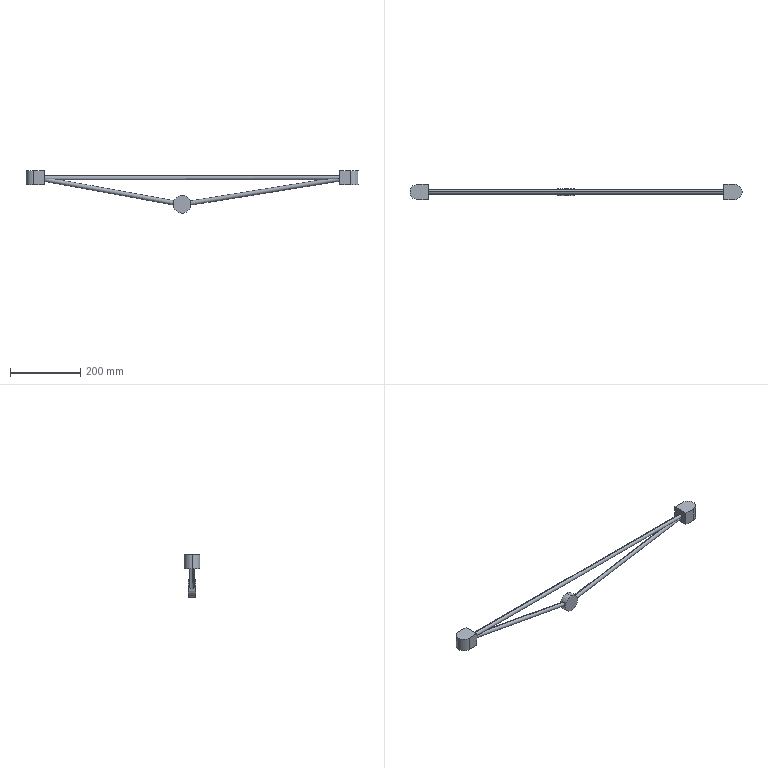Part | SolidWorks | features MoveFace 4, BaseBody 2, Sweep 1 | 1 solid | 23 faces | box 944 x 44 x 120.397 mm | volume 388537 mm3 | plane 12 | cylinder 11 | commonest cylinder face diameters 12 x6 44 x3 50 x2
STEP:
#1=CARTESIAN_POINT('',(546.798,0.,-77.466));
#2=VERTEX_POINT('',#1);
#3=CARTESIAN_POINT('',(544.892,0.,-65.619));
#4=VERTEX_POINT('',#3);
#5=CARTESIAN_POINT('',(546.798,0.,-77.466));
#6=CARTESIAN_POINT('',(546.798,0.398,-77.466));
#7=CARTESIAN_POINT('',(546.801,0.7891,-77.426));
#8=CARTESIAN_POINT('',(546.81,1.366,-77.308));
#9=CARTESIAN_POINT('',(546.814,1.556,-77.259));
#10=CARTESIAN_POINT('',(546.823,1.934,-77.142));
#11=CARTESIAN_POINT('',(546.827,2.121,-77.073));
#12=CARTESIAN_POINT('',(546.842,2.666,-76.841));
#13=CARTESIAN_POINT('',(546.853,3.01,-76.653));
#14=CARTESIAN_POINT('',(546.871,3.661,-76.209));
#15=CARTESIAN_POINT('',(546.879,3.968,-75.952));
#16=CARTESIAN_POINT('',(546.885,4.519,-75.392));
#17=CARTESIAN_POINT('',(546.884,4.767,-75.087));
#18=CARTESIAN_POINT('',(546.867,5.206,-74.426));
#19=CARTESIAN_POINT('',(546.851,5.391,-74.077));
#20=CARTESIAN_POINT('',(546.815,5.616,-73.535));
#21=CARTESIAN_POINT('',(546.8,5.682,-73.351));
#22=CARTESIAN_POINT('',(546.767,5.797,-72.975));
#23=CARTESIAN_POINT('',(546.747,5.845,-72.782));
#24=CARTESIAN_POINT('',(546.682,5.961,-72.204));
#25=CARTESIAN_POINT('',(546.629,6.,-71.817));
#26=CARTESIAN_POINT('',(546.504,6.,-71.041));
#27=CARTESIAN_POINT('',(546.431,5.961,-70.648));
#28=CARTESIAN_POINT('',(546.273,5.807,-69.893));
#29=CARTESIAN_POINT('',(546.187,5.693,-69.527));
#30=CARTESIAN_POINT('',(546.051,5.466,-68.996));
#31=CARTESIAN_POINT('',(546.004,5.381,-68.822));
#32=CARTESIAN_POINT('',(545.91,5.196,-68.486));
#33=CARTESIAN_POINT('',(545.863,5.095,-68.324));
#34=CARTESIAN_POINT('',(545.768,4.878,-68.011));
#35=CARTESIAN_POINT('',(545.721,4.762,-67.86));
#36=CARTESIAN_POINT('',(545.627,4.513,-67.569));
#37=CARTESIAN_POINT('',(545.58,4.381,-67.428));
#38=CARTESIAN_POINT('',(545.443,3.963,-67.027));
#39=CARTESIAN_POINT('',(545.357,3.662,-66.791));
#40=CARTESIAN_POINT('',(545.2,3.013,-66.376));
#41=CARTESIAN_POINT('',(545.13,2.662,-66.197));
#42=CARTESIAN_POINT('',(545.014,1.937,-65.911));
#43=CARTESIAN_POINT('',(544.969,1.563,-65.803));
#44=CARTESIAN_POINT('',(544.923,0.9839,-65.693));
#45=CARTESIAN_POINT('',(544.911,0.7866,-65.665));
#46=CARTESIAN_POINT('',(544.896,0.3928,-65.628));
#47=CARTESIAN_POINT('',(544.892,0.1962,-65.619));
#48=CARTESIAN_POINT('',(544.892,0.,-65.619));
#49=B_SPLINE_CURVE_WITH_KNOTS('',3,(#5,#6,#7,#8,#9,#10,#11,#12,#13,#14,#15,#16,#17,#18,#19,#20,#21,#22,#23,#24,#25,#26,#27,#28,#29,#30,#31,#32,#33,#34,#35,#36,#37,#38,#39,#40,#41,#42,#43,#44,#45,#46,#47,#48),.UNSPECIFIED.,.F.,.F.,(4,2,2,2,2,2,2,2,2,2,2,2,2,2,2,2,2,2,2,2,2,4),(0.,0.001177,0.001765,0.002353,0.00353,0.004707,0.005884,0.00706,0.007649,0.008237,0.009414,0.01059,0.01177,0.01236,0.01294,0.01353,0.01412,0.0153,0.01647,0.01765,0.01824,0.01883),.UNSPECIFIED.);
#50=EDGE_CURVE('',#2,#4,#49,.T.);
#51=ORIENTED_EDGE('',*,*,#50,.F.);
#52=CARTESIAN_POINT('',(544.892,0.,-65.619));
#53=CARTESIAN_POINT('',(544.892,-0.3923,-65.619));
#54=CARTESIAN_POINT('',(544.907,-0.7833,-65.655));
#55=CARTESIAN_POINT('',(544.969,-1.562,-65.802));
#56=CARTESIAN_POINT('',(545.015,-1.938,-65.911));
#57=CARTESIAN_POINT('',(545.101,-2.48,-66.125));
#58=CARTESIAN_POINT('',(545.132,-2.657,-66.205));
#59=CARTESIAN_POINT('',(545.202,-3.004,-66.382));
#60=CARTESIAN_POINT('',(545.239,-3.174,-66.479));
#61=CARTESIAN_POINT('',(545.357,-3.663,-66.791));
#62=CARTESIAN_POINT('',(545.443,-3.964,-67.028));
#63=CARTESIAN_POINT('',(545.625,-4.517,-67.559));
#64=CARTESIAN_POINT('',(545.721,-4.769,-67.854));
#65=CARTESIAN_POINT('',(545.91,-5.203,-68.481));
#66=CARTESIAN_POINT('',(546.004,-5.388,-68.814));
#67=CARTESIAN_POINT('',(546.187,-5.692,-69.523));
#68=CARTESIAN_POINT('',(546.273,-5.807,-69.892));
#69=CARTESIAN_POINT('',(546.391,-5.922,-70.457));
#70=CARTESIAN_POINT('',(546.429,-5.951,-70.647));
#71=CARTESIAN_POINT('',(546.5,-5.99,-71.033));
#72=CARTESIAN_POINT('',(546.534,-6.,-71.229));
#73=CARTESIAN_POINT('',(546.629,-6.,-71.815));
#74=CARTESIAN_POINT('',(546.682,-5.961,-72.202));
#75=CARTESIAN_POINT('',(546.768,-5.808,-72.968));
#76=CARTESIAN_POINT('',(546.802,-5.692,-73.351));
#77=CARTESIAN_POINT('',(546.851,-5.392,-74.076));
#78=CARTESIAN_POINT('',(546.867,-5.208,-74.423));
#79=CARTESIAN_POINT('',(546.879,-4.88,-74.917));
#80=CARTESIAN_POINT('',(546.882,-4.762,-75.078));
#81=CARTESIAN_POINT('',(546.884,-4.513,-75.385));
#82=CARTESIAN_POINT('',(546.884,-4.382,-75.531));
#83=CARTESIAN_POINT('',(546.879,-3.97,-75.95));
#84=CARTESIAN_POINT('',(546.871,-3.666,-76.205));
#85=CARTESIAN_POINT('',(546.853,-3.011,-76.652));
#86=CARTESIAN_POINT('',(546.842,-2.667,-76.84));
#87=CARTESIAN_POINT('',(546.823,-1.945,-77.148));
#88=CARTESIAN_POINT('',(546.814,-1.564,-77.268));
#89=CARTESIAN_POINT('',(546.801,-0.7902,-77.426));
#90=CARTESIAN_POINT('',(546.798,-0.3979,-77.466));
#91=CARTESIAN_POINT('',(546.798,0.,-77.466));
#92=B_SPLINE_CURVE_WITH_KNOTS('',3,(#52,#53,#54,#55,#56,#57,#58,#59,#60,#61,#62,#63,#64,#65,#66,#67,#68,#69,#70,#71,#72,#73,#74,#75,#76,#77,#78,#79,#80,#81,#82,#83,#84,#85,#86,#87,#88,#89,#90,#91),.UNSPECIFIED.,.F.,.F.,(4,2,2,2,2,2,2,2,2,2,2,2,2,2,2,2,2,2,2,4),(0.01883,0.02,0.02118,0.02177,0.02236,0.02353,0.02471,0.02589,0.02706,0.02765,0.02824,0.02942,0.03059,0.03177,0.03236,0.03294,0.03412,0.0353,0.03647,0.03765),.UNSPECIFIED.);
#93=EDGE_CURVE('',#4,#2,#92,.T.);
#94=ORIENTED_EDGE('',*,*,#93,.F.);
#95=EDGE_LOOP('',(#51,#94));
#96=FACE_BOUND('',#95,.T.);
#97=CARTESIAN_POINT('',(521.883,10.,-50.397));
#98=VERTEX_POINT('',#97);
#99=CARTESIAN_POINT('',(521.883,10.,-100.397));
#100=VERTEX_POINT('',#99);
#101=CARTESIAN_POINT('',(521.883,10.,-75.397));
#102=DIRECTION('',(0.,1.,0.));
#103=DIRECTION('',(0.,0.,-1.));
#104=AXIS2_PLACEMENT_3D('',#101,#102,#103);
#105=CIRCLE('',#104,25.);
#106=EDGE_CURVE('',#98,#100,#105,.T.);
#107=ORIENTED_EDGE('',*,*,#106,.F.);
#108=CARTESIAN_POINT('',(521.883,-10.,-50.397));
#109=VERTEX_POINT('',#108);
#110=CARTESIAN_POINT('',(521.883,10.,-50.397));
#111=DIRECTION('',(0.,-1.,0.));
#112=VECTOR('',#111,1000.);
#113=LINE('',#110,#112);
#114=EDGE_CURVE('',#98,#109,#113,.T.);
#115=ORIENTED_EDGE('',*,*,#114,.T.);
#116=CARTESIAN_POINT('',(521.883,-10.,-100.397));
#117=VERTEX_POINT('',#116);
#118=CARTESIAN_POINT('',(521.883,-10.,-75.397));
#119=DIRECTION('',(0.,1.,0.));
#120=DIRECTION('',(0.,0.,-1.));
#121=AXIS2_PLACEMENT_3D('',#118,#119,#120);
#122=CIRCLE('',#121,25.);
#123=EDGE_CURVE('',#109,#117,#122,.T.);
#124=ORIENTED_EDGE('',*,*,#123,.T.);
#125=CARTESIAN_POINT('',(521.883,10.,-100.397));
#126=DIRECTION('',(0.,-1.,0.));
#127=VECTOR('',#126,1000.);
#128=LINE('',#125,#127);
#129=EDGE_CURVE('',#100,#117,#128,.T.);
#130=ORIENTED_EDGE('',*,*,#129,.F.);
#131=EDGE_LOOP('',(#107,#115,#124,#130));
#132=FACE_OUTER_BOUND('',#131,.T.);
#133=CARTESIAN_POINT('',(521.883,10.,-75.397));
#134=DIRECTION('',(0.,-1.,0.));
#135=DIRECTION('',(0.,0.,-1.));
#136=AXIS2_PLACEMENT_3D('',#133,#134,#135);
#137=CYLINDRICAL_SURFACE('',#136,25.);
#138=ADVANCED_FACE('',(#96,#132),#137,.T.);
#139=CARTESIAN_POINT('',(174.528,0.,-6.));
#140=VERTEX_POINT('',#139);
#141=CARTESIAN_POINT('',(130.,5.665,-1.976));
#142=VERTEX_POINT('',#141);
#143=CARTESIAN_POINT('',(174.528,0.,-6.));
#144=CARTESIAN_POINT('',(174.528,2.642,-6.));
#145=CARTESIAN_POINT('',(157.601,4.795,-4.47));
#146=CARTESIAN_POINT('',(130.,5.665,-1.976));
#147=(BOUNDED_CURVE()B_SPLINE_CURVE(3,(#143,#144,#145,#146),.UNSPECIFIED.,.F.,.F.)B_SPLINE_CURVE_WITH_KNOTS((4,4),(0.,1.235),.UNSPECIFIED.)CURVE()GEOMETRIC_REPRESENTATION_ITEM()RATIONAL_B_SPLINE_CURVE((1.,0.8768,0.8768,1.))REPRESENTATION_ITEM(''));
#148=EDGE_CURVE('',#140,#142,#147,.T.);
#149=ORIENTED_EDGE('',*,*,#148,.F.);
#150=CARTESIAN_POINT('',(499.083,0.,-65.143));
#151=VERTEX_POINT('',#150);
#152=CARTESIAN_POINT('',(109.21,0.,5.903));
#153=DIRECTION('',(0.9838,0.,-0.1793));
#154=VECTOR('',#153,1000.);
#155=LINE('',#152,#154);
#156=EDGE_CURVE('',#140,#151,#155,.T.);
#157=ORIENTED_EDGE('',*,*,#156,.T.);
#158=CARTESIAN_POINT('',(496.932,0.,-76.949));
#159=VERTEX_POINT('',#158);
#160=CARTESIAN_POINT('',(499.083,0.,-65.143));
#161=CARTESIAN_POINT('',(499.083,0.3923,-65.143));
#162=CARTESIAN_POINT('',(499.067,0.7833,-65.179));
#163=CARTESIAN_POINT('',(499.002,1.562,-65.325));
#164=CARTESIAN_POINT('',(498.954,1.938,-65.433));
#165=CARTESIAN_POINT('',(498.864,2.48,-65.645));
#166=CARTESIAN_POINT('',(498.83,2.657,-65.724));
#167=CARTESIAN_POINT('',(498.758,3.004,-65.899));
#168=CARTESIAN_POINT('',(498.718,3.174,-65.996));
#169=CARTESIAN_POINT('',(498.594,3.663,-66.306));
#170=CARTESIAN_POINT('',(498.503,3.964,-66.54));
#171=CARTESIAN_POINT('',(498.31,4.517,-67.067));
#172=CARTESIAN_POINT('',(498.208,4.769,-67.361));
#173=CARTESIAN_POINT('',(498.006,5.203,-67.983));
#174=CARTESIAN_POINT('',(497.905,5.388,-68.314));
#175=CARTESIAN_POINT('',(497.708,5.692,-69.02));
#176=CARTESIAN_POINT('',(497.614,5.807,-69.387));
#177=CARTESIAN_POINT('',(497.484,5.922,-69.949));
#178=CARTESIAN_POINT('',(497.442,5.951,-70.138));
#179=CARTESIAN_POINT('',(497.362,5.99,-70.522));
#180=CARTESIAN_POINT('',(497.324,6.,-70.718));
#181=CARTESIAN_POINT('',(497.218,6.,-71.302));
#182=CARTESIAN_POINT('',(497.157,5.961,-71.688));
#183=CARTESIAN_POINT('',(497.055,5.808,-72.452));
#184=CARTESIAN_POINT('',(497.013,5.692,-72.834));
#185=CARTESIAN_POINT('',(496.949,5.392,-73.558));
#186=CARTESIAN_POINT('',(496.926,5.208,-73.904));
#187=CARTESIAN_POINT('',(496.903,4.88,-74.399));
#188=CARTESIAN_POINT('',(496.897,4.762,-74.559));
#189=CARTESIAN_POINT('',(496.889,4.513,-74.865));
#190=CARTESIAN_POINT('',(496.886,4.382,-75.012));
#191=CARTESIAN_POINT('',(496.882,3.97,-75.431));
#192=CARTESIAN_POINT('',(496.884,3.666,-75.686));
#193=CARTESIAN_POINT('',(496.893,3.011,-76.133));
#194=CARTESIAN_POINT('',(496.9,2.667,-76.322));
#195=CARTESIAN_POINT('',(496.913,1.945,-76.629));
#196=CARTESIAN_POINT('',(496.92,1.564,-76.749));
#197=CARTESIAN_POINT('',(496.929,0.7902,-76.908));
#198=CARTESIAN_POINT('',(496.932,0.3979,-76.949));
#199=CARTESIAN_POINT('',(496.932,0.,-76.949));
#200=B_SPLINE_CURVE_WITH_KNOTS('',3,(#160,#161,#162,#163,#164,#165,#166,#167,#168,#169,#170,#171,#172,#173,#174,#175,#176,#177,#178,#179,#180,#181,#182,#183,#184,#185,#186,#187,#188,#189,#190,#191,#192,#193,#194,#195,#196,#197,#198,#199),.UNSPECIFIED.,.F.,.F.,(4,2,2,2,2,2,2,2,2,2,2,2,2,2,2,2,2,2,2,4),(0.01883,0.02,0.02118,0.02177,0.02236,0.02353,0.02471,0.02589,0.02706,0.02765,0.02824,0.02942,0.03059,0.03177,0.03236,0.03294,0.03412,0.0353,0.03647,0.03765),.UNSPECIFIED.);
#201=EDGE_CURVE('',#151,#159,#200,.T.);
#202=ORIENTED_EDGE('',*,*,#201,.T.);
#203=CARTESIAN_POINT('',(130.,0.,-10.083));
#204=VERTEX_POINT('',#203);
#205=CARTESIAN_POINT('',(107.059,0.,-5.903));
#206=DIRECTION('',(0.9838,0.,-0.1793));
#207=VECTOR('',#206,1000.);
#208=LINE('',#205,#207);
#209=EDGE_CURVE('',#204,#159,#208,.T.);
#210=ORIENTED_EDGE('',*,*,#209,.F.);
#211=CARTESIAN_POINT('',(130.,0.,-10.083));
#212=CARTESIAN_POINT('',(130.,4.533,-10.083));
#213=CARTESIAN_POINT('',(130.,7.158,-6.327));
#214=CARTESIAN_POINT('',(130.,5.665,-1.976));
#215=(BOUNDED_CURVE()B_SPLINE_CURVE(3,(#211,#212,#213,#214),.UNSPECIFIED.,.F.,.F.)B_SPLINE_CURVE_WITH_KNOTS((4,4),(0.,1.906),.UNSPECIFIED.)CURVE()GEOMETRIC_REPRESENTATION_ITEM()RATIONAL_B_SPLINE_CURVE((1.,0.7194,0.7194,1.))REPRESENTATION_ITEM(''));
#216=EDGE_CURVE('',#204,#142,#215,.T.);
#217=ORIENTED_EDGE('',*,*,#216,.T.);
#218=EDGE_LOOP('',(#149,#157,#202,#210,#217));
#219=FACE_OUTER_BOUND('',#218,.T.);
#220=CARTESIAN_POINT('',(108.134,0.,0.));
#221=DIRECTION('',(0.9838,0.,-0.1793));
#222=DIRECTION('',(-0.1793,0.,-0.9838));
#223=AXIS2_PLACEMENT_3D('',#220,#221,#222);
#224=CYLINDRICAL_SURFACE('',#223,6.);
#225=ADVANCED_FACE('',(#219),#224,.T.);
#226=ORIENTED_EDGE('',*,*,#50,.T.);
#227=CARTESIAN_POINT('',(915.543,0.,-6.));
#228=VERTEX_POINT('',#227);
#229=CARTESIAN_POINT('',(519.714,0.,-69.669));
#230=DIRECTION('',(0.9873,0.,0.1588));
#231=VECTOR('',#230,1000.);
#232=LINE('',#229,#231);
#233=EDGE_CURVE('',#4,#228,#232,.T.);
#234=ORIENTED_EDGE('',*,*,#233,.T.);
#235=CARTESIAN_POINT('',(970.,5.769,-1.648));
#236=VERTEX_POINT('',#235);
#237=CARTESIAN_POINT('',(970.,5.769,-1.648));
#238=CARTESIAN_POINT('',(936.515,5.005,-4.324));
#239=CARTESIAN_POINT('',(915.543,2.783,-6.));
#240=CARTESIAN_POINT('',(915.543,0.,-6.));
#241=(BOUNDED_CURVE()B_SPLINE_CURVE(3,(#237,#238,#239,#240),.UNSPECIFIED.,.F.,.F.)B_SPLINE_CURVE_WITH_KNOTS((4,4),(1.849,3.142),.UNSPECIFIED.)CURVE()GEOMETRIC_REPRESENTATION_ITEM()RATIONAL_B_SPLINE_CURVE((1.,0.8656,0.8656,1.))REPRESENTATION_ITEM(''));
#242=EDGE_CURVE('',#236,#228,#241,.T.);
#243=ORIENTED_EDGE('',*,*,#242,.F.);
#244=CARTESIAN_POINT('',(970.,0.,-9.395));
#245=VERTEX_POINT('',#244);
#246=CARTESIAN_POINT('',(970.,5.769,-1.648));
#247=CARTESIAN_POINT('',(970.,6.963,-5.881));
#248=CARTESIAN_POINT('',(970.,4.346,-9.395));
#249=CARTESIAN_POINT('',(970.,0.,-9.395));
#250=(BOUNDED_CURVE()B_SPLINE_CURVE(3,(#246,#247,#248,#249),.UNSPECIFIED.,.F.,.F.)B_SPLINE_CURVE_WITH_KNOTS((4,4),(1.292,3.142),.UNSPECIFIED.)CURVE()GEOMETRIC_REPRESENTATION_ITEM()RATIONAL_B_SPLINE_CURVE((1.,0.7348,0.7348,1.))REPRESENTATION_ITEM(''));
#251=EDGE_CURVE('',#236,#245,#250,.T.);
#252=ORIENTED_EDGE('',*,*,#251,.T.);
#253=CARTESIAN_POINT('',(521.62,0.,-81.516));
#254=DIRECTION('',(0.9873,0.,0.1588));
#255=VECTOR('',#254,1000.);
#256=LINE('',#253,#255);
#257=EDGE_CURVE('',#2,#245,#256,.T.);
#258=ORIENTED_EDGE('',*,*,#257,.F.);
#259=EDGE_LOOP('',(#226,#234,#243,#252,#258));
#260=FACE_OUTER_BOUND('',#259,.T.);
#261=CARTESIAN_POINT('',(520.667,0.,-75.592));
#262=DIRECTION('',(0.9873,0.,0.1588));
#263=DIRECTION('',(0.1588,0.,-0.9873));
#264=AXIS2_PLACEMENT_3D('',#261,#262,#263);
#265=CYLINDRICAL_SURFACE('',#264,6.);
#266=ADVANCED_FACE('',(#260),#265,.T.);
#267=CARTESIAN_POINT('',(100.,-22.,20.));
#268=VERTEX_POINT('',#267);
#269=CARTESIAN_POINT('',(78.,0.,20.));
#270=VERTEX_POINT('',#269);
#271=CARTESIAN_POINT('',(100.,0.,20.));
#272=DIRECTION('',(0.,0.,-1.));
#273=DIRECTION('',(-1.,0.,0.));
#274=AXIS2_PLACEMENT_3D('',#271,#272,#273);
#275=CIRCLE('',#274,22.);
#276=EDGE_CURVE('',#268,#270,#275,.T.);
#277=ORIENTED_EDGE('',*,*,#276,.T.);
#278=CARTESIAN_POINT('',(78.,0.,-20.));
#279=VERTEX_POINT('',#278);
#280=CARTESIAN_POINT('',(78.,0.,10.));
#281=DIRECTION('',(0.,0.,-1.));
#282=VECTOR('',#281,1000.);
#283=LINE('',#280,#282);
#284=EDGE_CURVE('',#270,#279,#283,.T.);
#285=ORIENTED_EDGE('',*,*,#284,.T.);
#286=CARTESIAN_POINT('',(100.,-22.,-20.));
#287=VERTEX_POINT('',#286);
#288=CARTESIAN_POINT('',(100.,0.,-20.));
#289=DIRECTION('',(0.,0.,-1.));
#290=DIRECTION('',(-1.,0.,0.));
#291=AXIS2_PLACEMENT_3D('',#288,#289,#290);
#292=CIRCLE('',#291,22.);
#293=EDGE_CURVE('',#287,#279,#292,.T.);
#294=ORIENTED_EDGE('',*,*,#293,.F.);
#295=CARTESIAN_POINT('',(100.,-22.,10.));
#296=DIRECTION('',(0.,0.,1.));
#297=VECTOR('',#296,1000.);
#298=LINE('',#295,#297);
#299=EDGE_CURVE('',#287,#268,#298,.T.);
#300=ORIENTED_EDGE('',*,*,#299,.T.);
#301=EDGE_LOOP('',(#277,#285,#294,#300));
#302=FACE_OUTER_BOUND('',#301,.T.);
#303=CARTESIAN_POINT('',(100.,0.,10.));
#304=DIRECTION('',(0.,0.,-1.));
#305=DIRECTION('',(-1.,0.,0.));
#306=AXIS2_PLACEMENT_3D('',#303,#304,#305);
#307=CYLINDRICAL_SURFACE('',#306,22.);
#308=ADVANCED_FACE('',(#302),#307,.T.);
#309=CARTESIAN_POINT('',(130.,0.,6.));
#310=VERTEX_POINT('',#309);
#311=CARTESIAN_POINT('',(130.,0.,0.));
#312=DIRECTION('',(1.,0.,0.));
#313=DIRECTION('',(0.,0.,1.));
#314=AXIS2_PLACEMENT_3D('',#311,#312,#313);
#315=CIRCLE('',#314,6.);
#316=EDGE_CURVE('',#142,#310,#315,.T.);
#317=ORIENTED_EDGE('',*,*,#316,.T.);
#318=CARTESIAN_POINT('',(970.,0.,6.));
#319=VERTEX_POINT('',#318);
#320=CARTESIAN_POINT('',(100.,0.,6.));
#321=DIRECTION('',(1.,0.,0.));
#322=VECTOR('',#321,1000.);
#323=LINE('',#320,#322);
#324=EDGE_CURVE('',#310,#319,#323,.T.);
#325=ORIENTED_EDGE('',*,*,#324,.T.);
#326=CARTESIAN_POINT('',(970.,0.,0.));
#327=DIRECTION('',(-1.,0.,0.));
#328=DIRECTION('',(0.,0.,-1.));
#329=AXIS2_PLACEMENT_3D('',#326,#327,#328);
#330=CIRCLE('',#329,6.);
#331=EDGE_CURVE('',#319,#236,#330,.T.);
#332=ORIENTED_EDGE('',*,*,#331,.T.);
#333=ORIENTED_EDGE('',*,*,#242,.T.);
#334=CARTESIAN_POINT('',(100.,0.,-6.));
#335=DIRECTION('',(1.,0.,0.));
#336=VECTOR('',#335,1000.);
#337=LINE('',#334,#336);
#338=EDGE_CURVE('',#140,#228,#337,.T.);
#339=ORIENTED_EDGE('',*,*,#338,.F.);
#340=ORIENTED_EDGE('',*,*,#148,.T.);
#341=EDGE_LOOP('',(#317,#325,#332,#333,#339,#340));
#342=FACE_OUTER_BOUND('',#341,.T.);
#343=CARTESIAN_POINT('',(100.,0.,0.));
#344=DIRECTION('',(1.,0.,0.));
#345=DIRECTION('',(0.,0.,-1.));
#346=AXIS2_PLACEMENT_3D('',#343,#344,#345);
#347=CYLINDRICAL_SURFACE('',#346,6.);
#348=ADVANCED_FACE('',(#342),#347,.T.);
#349=ORIENTED_EDGE('',*,*,#324,.F.);
#350=CARTESIAN_POINT('',(130.,-5.665,-1.976));
#351=VERTEX_POINT('',#350);
#352=CARTESIAN_POINT('',(130.,0.,0.));
#353=DIRECTION('',(1.,0.,0.));
#354=DIRECTION('',(0.,0.,1.));
#355=AXIS2_PLACEMENT_3D('',#352,#353,#354);
#356=CIRCLE('',#355,6.);
#357=EDGE_CURVE('',#310,#351,#356,.T.);
#358=ORIENTED_EDGE('',*,*,#357,.T.);
#359=CARTESIAN_POINT('',(130.,-5.665,-1.976));
#360=CARTESIAN_POINT('',(157.601,-4.795,-4.47));
#361=CARTESIAN_POINT('',(174.528,-2.642,-6.));
#362=CARTESIAN_POINT('',(174.528,0.,-6.));
#363=(BOUNDED_CURVE()B_SPLINE_CURVE(3,(#359,#360,#361,#362),.UNSPECIFIED.,.F.,.F.)B_SPLINE_CURVE_WITH_KNOTS((4,4),(5.048,6.283),.UNSPECIFIED.)CURVE()GEOMETRIC_REPRESENTATION_ITEM()RATIONAL_B_SPLINE_CURVE((1.,0.8768,0.8768,1.))REPRESENTATION_ITEM(''));
#364=EDGE_CURVE('',#351,#140,#363,.T.);
#365=ORIENTED_EDGE('',*,*,#364,.T.);
#366=ORIENTED_EDGE('',*,*,#338,.T.);
#367=CARTESIAN_POINT('',(970.,-5.769,-1.648));
#368=VERTEX_POINT('',#367);
#369=CARTESIAN_POINT('',(915.543,0.,-6.));
#370=CARTESIAN_POINT('',(915.543,-2.783,-6.));
#371=CARTESIAN_POINT('',(936.515,-5.005,-4.324));
#372=CARTESIAN_POINT('',(970.,-5.769,-1.648));
#373=(BOUNDED_CURVE()B_SPLINE_CURVE(3,(#369,#370,#371,#372),.UNSPECIFIED.,.F.,.F.)B_SPLINE_CURVE_WITH_KNOTS((4,4),(3.142,4.434),.UNSPECIFIED.)CURVE()GEOMETRIC_REPRESENTATION_ITEM()RATIONAL_B_SPLINE_CURVE((1.,0.8656,0.8656,1.))REPRESENTATION_ITEM(''));
#374=EDGE_CURVE('',#228,#368,#373,.T.);
#375=ORIENTED_EDGE('',*,*,#374,.T.);
#376=CARTESIAN_POINT('',(970.,0.,0.));
#377=DIRECTION('',(-1.,0.,0.));
#378=DIRECTION('',(0.,0.,-1.));
#379=AXIS2_PLACEMENT_3D('',#376,#377,#378);
#380=CIRCLE('',#379,6.);
#381=EDGE_CURVE('',#368,#319,#380,.T.);
#382=ORIENTED_EDGE('',*,*,#381,.T.);
#383=EDGE_LOOP('',(#349,#358,#365,#366,#375,#382));
#384=FACE_OUTER_BOUND('',#383,.T.);
#385=CARTESIAN_POINT('',(100.,0.,0.));
#386=DIRECTION('',(1.,0.,0.));
#387=DIRECTION('',(0.,0.,-1.));
#388=AXIS2_PLACEMENT_3D('',#385,#386,#387);
#389=CYLINDRICAL_SURFACE('',#388,6.);
#390=ADVANCED_FACE('',(#384),#389,.T.);
#391=ORIENTED_EDGE('',*,*,#251,.F.);
#392=ORIENTED_EDGE('',*,*,#331,.F.);
#393=ORIENTED_EDGE('',*,*,#381,.F.);
#394=CARTESIAN_POINT('',(970.,0.,-9.395));
#395=CARTESIAN_POINT('',(970.,-4.346,-9.395));
#396=CARTESIAN_POINT('',(970.,-6.963,-5.881));
#397=CARTESIAN_POINT('',(970.,-5.769,-1.648));
#398=(BOUNDED_CURVE()B_SPLINE_CURVE(3,(#394,#395,#396,#397),.UNSPECIFIED.,.F.,.F.)B_SPLINE_CURVE_WITH_KNOTS((4,4),(3.142,4.991),.UNSPECIFIED.)CURVE()GEOMETRIC_REPRESENTATION_ITEM()RATIONAL_B_SPLINE_CURVE((1.,0.7348,0.7348,1.))REPRESENTATION_ITEM(''));
#399=EDGE_CURVE('',#245,#368,#398,.T.);
#400=ORIENTED_EDGE('',*,*,#399,.F.);
#401=EDGE_LOOP('',(#391,#392,#393,#400));
#402=FACE_BOUND('',#401,.T.);
#403=CARTESIAN_POINT('',(970.,-22.,20.));
#404=VERTEX_POINT('',#403);
#405=CARTESIAN_POINT('',(970.,-22.,-20.));
#406=VERTEX_POINT('',#405);
#407=CARTESIAN_POINT('',(970.,-22.,10.));
#408=DIRECTION('',(0.,0.,-1.));
#409=VECTOR('',#408,1000.);
#410=LINE('',#407,#409);
#411=EDGE_CURVE('',#404,#406,#410,.T.);
#412=ORIENTED_EDGE('',*,*,#411,.F.);
#413=CARTESIAN_POINT('',(970.,22.,20.));
#414=VERTEX_POINT('',#413);
#415=CARTESIAN_POINT('',(970.,12.,20.));
#416=DIRECTION('',(0.,-1.,0.));
#417=VECTOR('',#416,1000.);
#418=LINE('',#415,#417);
#419=EDGE_CURVE('',#414,#404,#418,.T.);
#420=ORIENTED_EDGE('',*,*,#419,.F.);
#421=CARTESIAN_POINT('',(970.,22.,-20.));
#422=VERTEX_POINT('',#421);
#423=CARTESIAN_POINT('',(970.,22.,10.));
#424=DIRECTION('',(0.,0.,1.));
#425=VECTOR('',#424,1000.);
#426=LINE('',#423,#425);
#427=EDGE_CURVE('',#422,#414,#426,.T.);
#428=ORIENTED_EDGE('',*,*,#427,.F.);
#429=CARTESIAN_POINT('',(970.,0.,-20.));
#430=DIRECTION('',(0.,1.,0.));
#431=VECTOR('',#430,1000.);
#432=LINE('',#429,#431);
#433=EDGE_CURVE('',#406,#422,#432,.T.);
#434=ORIENTED_EDGE('',*,*,#433,.F.);
#435=EDGE_LOOP('',(#412,#420,#428,#434));
#436=FACE_OUTER_BOUND('',#435,.T.);
#437=CARTESIAN_POINT('',(970.,12.,10.));
#438=DIRECTION('',(1.,0.,0.));
#439=DIRECTION('',(0.,0.,-1.));
#440=AXIS2_PLACEMENT_3D('',#437,#438,#439);
#441=PLANE('',#440);
#442=ADVANCED_FACE('',(#402,#436),#441,.F.);
#443=CARTESIAN_POINT('',(130.,-5.665,-1.976));
#444=CARTESIAN_POINT('',(130.,-7.158,-6.327));
#445=CARTESIAN_POINT('',(130.,-4.533,-10.083));
#446=CARTESIAN_POINT('',(130.,0.,-10.083));
#447=(BOUNDED_CURVE()B_SPLINE_CURVE(3,(#443,#444,#445,#446),.UNSPECIFIED.,.F.,.F.)B_SPLINE_CURVE_WITH_KNOTS((4,4),(4.377,6.283),.UNSPECIFIED.)CURVE()GEOMETRIC_REPRESENTATION_ITEM()RATIONAL_B_SPLINE_CURVE((1.,0.7194,0.7194,1.))REPRESENTATION_ITEM(''));
#448=EDGE_CURVE('',#351,#204,#447,.T.);
#449=ORIENTED_EDGE('',*,*,#448,.F.);
#450=ORIENTED_EDGE('',*,*,#357,.F.);
#451=ORIENTED_EDGE('',*,*,#316,.F.);
#452=ORIENTED_EDGE('',*,*,#216,.F.);
#453=EDGE_LOOP('',(#449,#450,#451,#452));
#454=FACE_BOUND('',#453,.T.);
#455=CARTESIAN_POINT('',(130.,22.,20.));
#456=VERTEX_POINT('',#455);
#457=CARTESIAN_POINT('',(130.,22.,-20.));
#458=VERTEX_POINT('',#457);
#459=CARTESIAN_POINT('',(130.,22.,10.));
#460=DIRECTION('',(0.,0.,-1.));
#461=VECTOR('',#460,1000.);
#462=LINE('',#459,#461);
#463=EDGE_CURVE('',#456,#458,#462,.T.);
#464=ORIENTED_EDGE('',*,*,#463,.F.);
#465=CARTESIAN_POINT('',(130.,-22.,20.));
#466=VERTEX_POINT('',#465);
#467=CARTESIAN_POINT('',(130.,0.,20.));
#468=DIRECTION('',(0.,1.,0.));
#469=VECTOR('',#468,1000.);
#470=LINE('',#467,#469);
#471=EDGE_CURVE('',#466,#456,#470,.T.);
#472=ORIENTED_EDGE('',*,*,#471,.F.);
#473=CARTESIAN_POINT('',(130.,-22.,-20.));
#474=VERTEX_POINT('',#473);
#475=CARTESIAN_POINT('',(130.,-22.,10.));
#476=DIRECTION('',(0.,0.,1.));
#477=VECTOR('',#476,1000.);
#478=LINE('',#475,#477);
#479=EDGE_CURVE('',#474,#466,#478,.T.);
#480=ORIENTED_EDGE('',*,*,#479,.F.);
#481=CARTESIAN_POINT('',(130.,12.,-20.));
#482=DIRECTION('',(0.,-1.,0.));
#483=VECTOR('',#482,1000.);
#484=LINE('',#481,#483);
#485=EDGE_CURVE('',#458,#474,#484,.T.);
#486=ORIENTED_EDGE('',*,*,#485,.F.);
#487=EDGE_LOOP('',(#464,#472,#480,#486));
#488=FACE_OUTER_BOUND('',#487,.T.);
#489=CARTESIAN_POINT('',(130.,12.,10.));
#490=DIRECTION('',(-1.,0.,0.));
#491=DIRECTION('',(0.,0.,1.));
#492=AXIS2_PLACEMENT_3D('',#489,#490,#491);
#493=PLANE('',#492);
#494=ADVANCED_FACE('',(#454,#488),#493,.F.);
#495=CARTESIAN_POINT('',(1000.,-22.,-20.));
#496=VERTEX_POINT('',#495);
#497=CARTESIAN_POINT('',(1000.,-22.,-20.));
#498=DIRECTION('',(1.,0.,0.));
#499=VECTOR('',#498,1000.);
#500=LINE('',#497,#499);
#501=EDGE_CURVE('',#406,#496,#500,.T.);
#502=ORIENTED_EDGE('',*,*,#501,.F.);
#503=ORIENTED_EDGE('',*,*,#433,.T.);
#504=CARTESIAN_POINT('',(1000.,22.,-20.));
#505=VERTEX_POINT('',#504);
#506=CARTESIAN_POINT('',(1000.,22.,-20.));
#507=DIRECTION('',(-1.,0.,0.));
#508=VECTOR('',#507,1000.);
#509=LINE('',#506,#508);
#510=EDGE_CURVE('',#505,#422,#509,.T.);
#511=ORIENTED_EDGE('',*,*,#510,.F.);
#512=CARTESIAN_POINT('',(1000.,0.,-20.));
#513=DIRECTION('',(0.,0.,1.));
#514=DIRECTION('',(1.,0.,0.));
#515=AXIS2_PLACEMENT_3D('',#512,#513,#514);
#516=CIRCLE('',#515,22.);
#517=EDGE_CURVE('',#496,#505,#516,.T.);
#518=ORIENTED_EDGE('',*,*,#517,.F.);
#519=EDGE_LOOP('',(#502,#503,#511,#518));
#520=FACE_OUTER_BOUND('',#519,.T.);
#521=CARTESIAN_POINT('',(1000.,0.,-20.));
#522=DIRECTION('',(0.,0.,1.));
#523=DIRECTION('',(1.,0.,0.));
#524=AXIS2_PLACEMENT_3D('',#521,#522,#523);
#525=PLANE('',#524);
#526=ADVANCED_FACE('',(#520),#525,.F.);
#527=CARTESIAN_POINT('',(1000.,-22.,20.));
#528=VERTEX_POINT('',#527);
#529=CARTESIAN_POINT('',(1000.,-22.,10.));
#530=DIRECTION('',(0.,0.,-1.));
#531=VECTOR('',#530,1000.);
#532=LINE('',#529,#531);
#533=EDGE_CURVE('',#528,#496,#532,.T.);
#534=ORIENTED_EDGE('',*,*,#533,.F.);
#535=CARTESIAN_POINT('',(1000.,-22.,20.));
#536=DIRECTION('',(1.,0.,0.));
#537=VECTOR('',#536,1000.);
#538=LINE('',#535,#537);
#539=EDGE_CURVE('',#404,#528,#538,.T.);
#540=ORIENTED_EDGE('',*,*,#539,.F.);
#541=ORIENTED_EDGE('',*,*,#411,.T.);
#542=ORIENTED_EDGE('',*,*,#501,.T.);
#543=EDGE_LOOP('',(#534,#540,#541,#542));
#544=FACE_OUTER_BOUND('',#543,.T.);
#545=CARTESIAN_POINT('',(1000.,-22.,10.));
#546=DIRECTION('',(0.,1.,0.));
#547=DIRECTION('',(-1.,0.,0.));
#548=AXIS2_PLACEMENT_3D('',#545,#546,#547);
#549=PLANE('',#548);
#550=ADVANCED_FACE('',(#544),#549,.F.);
#551=ORIENTED_EDGE('',*,*,#419,.T.);
#552=ORIENTED_EDGE('',*,*,#539,.T.);
#553=CARTESIAN_POINT('',(1000.,22.,20.));
#554=VERTEX_POINT('',#553);
#555=CARTESIAN_POINT('',(1000.,0.,20.));
#556=DIRECTION('',(0.,0.,1.));
#557=DIRECTION('',(1.,0.,0.));
#558=AXIS2_PLACEMENT_3D('',#555,#556,#557);
#559=CIRCLE('',#558,22.);
#560=EDGE_CURVE('',#528,#554,#559,.T.);
#561=ORIENTED_EDGE('',*,*,#560,.T.);
#562=CARTESIAN_POINT('',(1000.,22.,20.));
#563=DIRECTION('',(-1.,0.,0.));
#564=VECTOR('',#563,1000.);
#565=LINE('',#562,#564);
#566=EDGE_CURVE('',#554,#414,#565,.T.);
#567=ORIENTED_EDGE('',*,*,#566,.T.);
#568=EDGE_LOOP('',(#551,#552,#561,#567));
#569=FACE_OUTER_BOUND('',#568,.T.);
#570=CARTESIAN_POINT('',(1000.,0.,20.));
#571=DIRECTION('',(0.,0.,1.));
#572=DIRECTION('',(1.,0.,0.));
#573=AXIS2_PLACEMENT_3D('',#570,#571,#572);
#574=PLANE('',#573);
#575=ADVANCED_FACE('',(#569),#574,.T.);
#576=ORIENTED_EDGE('',*,*,#427,.T.);
#577=ORIENTED_EDGE('',*,*,#566,.F.);
#578=CARTESIAN_POINT('',(1000.,22.,10.));
#579=DIRECTION('',(0.,0.,1.));
#580=VECTOR('',#579,1000.);
#581=LINE('',#578,#580);
#582=EDGE_CURVE('',#505,#554,#581,.T.);
#583=ORIENTED_EDGE('',*,*,#582,.F.);
#584=ORIENTED_EDGE('',*,*,#510,.T.);
#585=EDGE_LOOP('',(#576,#577,#583,#584));
#586=FACE_OUTER_BOUND('',#585,.T.);
#587=CARTESIAN_POINT('',(1000.,22.,10.));
#588=DIRECTION('',(0.,-1.,0.));
#589=DIRECTION('',(1.,0.,0.));
#590=AXIS2_PLACEMENT_3D('',#587,#588,#589);
#591=PLANE('',#590);
#592=ADVANCED_FACE('',(#586),#591,.F.);
#593=CARTESIAN_POINT('',(100.,-22.,-20.));
#594=DIRECTION('',(-1.,0.,0.));
#595=VECTOR('',#594,1000.);
#596=LINE('',#593,#595);
#597=EDGE_CURVE('',#474,#287,#596,.T.);
#598=ORIENTED_EDGE('',*,*,#597,.T.);
#599=ORIENTED_EDGE('',*,*,#293,.T.);
#600=CARTESIAN_POINT('',(100.,22.,-20.));
#601=VERTEX_POINT('',#600);
#602=CARTESIAN_POINT('',(100.,0.,-20.));
#603=DIRECTION('',(0.,0.,-1.));
#604=DIRECTION('',(-1.,0.,0.));
#605=AXIS2_PLACEMENT_3D('',#602,#603,#604);
#606=CIRCLE('',#605,22.);
#607=EDGE_CURVE('',#279,#601,#606,.T.);
#608=ORIENTED_EDGE('',*,*,#607,.T.);
#609=CARTESIAN_POINT('',(100.,22.,-20.));
#610=DIRECTION('',(1.,0.,0.));
#611=VECTOR('',#610,1000.);
#612=LINE('',#609,#611);
#613=EDGE_CURVE('',#601,#458,#612,.T.);
#614=ORIENTED_EDGE('',*,*,#613,.T.);
#615=ORIENTED_EDGE('',*,*,#485,.T.);
#616=EDGE_LOOP('',(#598,#599,#608,#614,#615));
#617=FACE_OUTER_BOUND('',#616,.T.);
#618=CARTESIAN_POINT('',(100.,0.,-20.));
#619=DIRECTION('',(0.,0.,-1.));
#620=DIRECTION('',(-1.,0.,0.));
#621=AXIS2_PLACEMENT_3D('',#618,#619,#620);
#622=PLANE('',#621);
#623=ADVANCED_FACE('',(#617),#622,.T.);
#624=CARTESIAN_POINT('',(100.,22.,20.));
#625=VERTEX_POINT('',#624);
#626=CARTESIAN_POINT('',(100.,22.,10.));
#627=DIRECTION('',(0.,0.,-1.));
#628=VECTOR('',#627,1000.);
#629=LINE('',#626,#628);
#630=EDGE_CURVE('',#625,#601,#629,.T.);
#631=ORIENTED_EDGE('',*,*,#630,.F.);
#632=CARTESIAN_POINT('',(100.,22.,20.));
#633=DIRECTION('',(-1.,0.,0.));
#634=VECTOR('',#633,1000.);
#635=LINE('',#632,#634);
#636=EDGE_CURVE('',#456,#625,#635,.T.);
#637=ORIENTED_EDGE('',*,*,#636,.F.);
#638=ORIENTED_EDGE('',*,*,#463,.T.);
#639=ORIENTED_EDGE('',*,*,#613,.F.);
#640=EDGE_LOOP('',(#631,#637,#638,#639));
#641=FACE_OUTER_BOUND('',#640,.T.);
#642=CARTESIAN_POINT('',(100.,22.,10.));
#643=DIRECTION('',(0.,-1.,0.));
#644=DIRECTION('',(0.,0.,-1.));
#645=AXIS2_PLACEMENT_3D('',#642,#643,#644);
#646=PLANE('',#645);
#647=ADVANCED_FACE('',(#641),#646,.F.);
#648=ORIENTED_EDGE('',*,*,#276,.F.);
#649=CARTESIAN_POINT('',(100.,-22.,20.));
#650=DIRECTION('',(-1.,0.,0.));
#651=VECTOR('',#650,1000.);
#652=LINE('',#649,#651);
#653=EDGE_CURVE('',#466,#268,#652,.T.);
#654=ORIENTED_EDGE('',*,*,#653,.F.);
#655=ORIENTED_EDGE('',*,*,#471,.T.);
#656=ORIENTED_EDGE('',*,*,#636,.T.);
#657=CARTESIAN_POINT('',(100.,0.,20.));
#658=DIRECTION('',(0.,0.,-1.));
#659=DIRECTION('',(-1.,0.,0.));
#660=AXIS2_PLACEMENT_3D('',#657,#658,#659);
#661=CIRCLE('',#660,22.);
#662=EDGE_CURVE('',#270,#625,#661,.T.);
#663=ORIENTED_EDGE('',*,*,#662,.F.);
#664=EDGE_LOOP('',(#648,#654,#655,#656,#663));
#665=FACE_OUTER_BOUND('',#664,.T.);
#666=CARTESIAN_POINT('',(100.,0.,20.));
#667=DIRECTION('',(0.,0.,-1.));
#668=DIRECTION('',(-1.,0.,0.));
#669=AXIS2_PLACEMENT_3D('',#666,#667,#668);
#670=PLANE('',#669);
#671=ADVANCED_FACE('',(#665),#670,.F.);
#672=ORIENTED_EDGE('',*,*,#479,.T.);
#673=ORIENTED_EDGE('',*,*,#653,.T.);
#674=ORIENTED_EDGE('',*,*,#299,.F.);
#675=ORIENTED_EDGE('',*,*,#597,.F.);
#676=EDGE_LOOP('',(#672,#673,#674,#675));
#677=FACE_OUTER_BOUND('',#676,.T.);
#678=CARTESIAN_POINT('',(100.,-22.,10.));
#679=DIRECTION('',(0.,1.,0.));
#680=DIRECTION('',(-1.,0.,0.));
#681=AXIS2_PLACEMENT_3D('',#678,#679,#680);
#682=PLANE('',#681);
#683=ADVANCED_FACE('',(#677),#682,.F.);
#684=ORIENTED_EDGE('',*,*,#560,.F.);
#685=ORIENTED_EDGE('',*,*,#533,.T.);
#686=ORIENTED_EDGE('',*,*,#517,.T.);
#687=ORIENTED_EDGE('',*,*,#582,.T.);
#688=EDGE_LOOP('',(#684,#685,#686,#687));
#689=FACE_OUTER_BOUND('',#688,.T.);
#690=CARTESIAN_POINT('',(1000.,0.,10.));
#691=DIRECTION('',(0.,0.,-1.));
#692=DIRECTION('',(-1.,0.,0.));
#693=AXIS2_PLACEMENT_3D('',#690,#691,#692);
#694=CYLINDRICAL_SURFACE('',#693,22.);
#695=ADVANCED_FACE('',(#689),#694,.T.);
#696=ORIENTED_EDGE('',*,*,#284,.F.);
#697=ORIENTED_EDGE('',*,*,#662,.T.);
#698=ORIENTED_EDGE('',*,*,#630,.T.);
#699=ORIENTED_EDGE('',*,*,#607,.F.);
#700=EDGE_LOOP('',(#696,#697,#698,#699));
#701=FACE_OUTER_BOUND('',#700,.T.);
#702=CARTESIAN_POINT('',(100.,0.,10.));
#703=DIRECTION('',(0.,0.,-1.));
#704=DIRECTION('',(-1.,0.,0.));
#705=AXIS2_PLACEMENT_3D('',#702,#703,#704);
#706=CYLINDRICAL_SURFACE('',#705,22.);
#707=ADVANCED_FACE('',(#701),#706,.T.);
#708=ORIENTED_EDGE('',*,*,#233,.F.);
#709=ORIENTED_EDGE('',*,*,#93,.T.);
#710=ORIENTED_EDGE('',*,*,#257,.T.);
#711=ORIENTED_EDGE('',*,*,#399,.T.);
#712=ORIENTED_EDGE('',*,*,#374,.F.);
#713=EDGE_LOOP('',(#708,#709,#710,#711,#712));
#714=FACE_OUTER_BOUND('',#713,.T.);
#715=CARTESIAN_POINT('',(520.667,0.,-75.592));
#716=DIRECTION('',(0.9873,0.,0.1588));
#717=DIRECTION('',(0.1588,0.,-0.9873));
#718=AXIS2_PLACEMENT_3D('',#715,#716,#717);
#719=CYLINDRICAL_SURFACE('',#718,6.);
#720=ADVANCED_FACE('',(#714),#719,.T.);
#721=ORIENTED_EDGE('',*,*,#156,.F.);
#722=ORIENTED_EDGE('',*,*,#364,.F.);
#723=ORIENTED_EDGE('',*,*,#448,.T.);
#724=ORIENTED_EDGE('',*,*,#209,.T.);
#725=CARTESIAN_POINT('',(496.932,0.,-76.949));
#726=CARTESIAN_POINT('',(496.932,-0.398,-76.949));
#727=CARTESIAN_POINT('',(496.929,-0.7891,-76.908));
#728=CARTESIAN_POINT('',(496.922,-1.366,-76.79));
#729=CARTESIAN_POINT('',(496.92,-1.556,-76.741));
#730=CARTESIAN_POINT('',(496.914,-1.934,-76.623));
#731=CARTESIAN_POINT('',(496.91,-2.121,-76.554));
#732=CARTESIAN_POINT('',(496.9,-2.666,-76.323));
#733=CARTESIAN_POINT('',(496.893,-3.01,-76.134));
#734=CARTESIAN_POINT('',(496.884,-3.661,-75.69));
#735=CARTESIAN_POINT('',(496.882,-3.968,-75.433));
#736=CARTESIAN_POINT('',(496.887,-4.519,-74.873));
#737=CARTESIAN_POINT('',(496.895,-4.767,-74.568));
#738=CARTESIAN_POINT('',(496.926,-5.206,-73.908));
#739=CARTESIAN_POINT('',(496.948,-5.391,-73.559));
#740=CARTESIAN_POINT('',(496.996,-5.616,-73.018));
#741=CARTESIAN_POINT('',(497.014,-5.682,-72.834));
#742=CARTESIAN_POINT('',(497.056,-5.797,-72.459));
#743=CARTESIAN_POINT('',(497.079,-5.845,-72.266));
#744=CARTESIAN_POINT('',(497.157,-5.961,-71.69));
#745=CARTESIAN_POINT('',(497.218,-6.,-71.304));
#746=CARTESIAN_POINT('',(497.358,-6.,-70.531));
#747=CARTESIAN_POINT('',(497.439,-5.961,-70.14));
#748=CARTESIAN_POINT('',(497.613,-5.807,-69.388));
#749=CARTESIAN_POINT('',(497.707,-5.693,-69.024));
#750=CARTESIAN_POINT('',(497.854,-5.466,-68.495));
#751=CARTESIAN_POINT('',(497.905,-5.381,-68.322));
#752=CARTESIAN_POINT('',(498.006,-5.196,-67.989));
#753=CARTESIAN_POINT('',(498.056,-5.095,-67.828));
#754=CARTESIAN_POINT('',(498.157,-4.878,-67.517));
#755=CARTESIAN_POINT('',(498.208,-4.762,-67.367));
#756=CARTESIAN_POINT('',(498.308,-4.513,-67.077));
#757=CARTESIAN_POINT('',(498.358,-4.381,-66.937));
#758=CARTESIAN_POINT('',(498.503,-3.963,-66.54));
#759=CARTESIAN_POINT('',(498.594,-3.662,-66.305));
#760=CARTESIAN_POINT('',(498.759,-3.013,-65.894));
#761=CARTESIAN_POINT('',(498.833,-2.662,-65.716));
#762=CARTESIAN_POINT('',(498.955,-1.937,-65.433));
#763=CARTESIAN_POINT('',(499.002,-1.563,-65.325));
#764=CARTESIAN_POINT('',(499.05,-0.9839,-65.216));
#765=CARTESIAN_POINT('',(499.063,-0.7866,-65.189));
#766=CARTESIAN_POINT('',(499.079,-0.3928,-65.152));
#767=CARTESIAN_POINT('',(499.083,-0.1962,-65.143));
#768=CARTESIAN_POINT('',(499.083,0.,-65.143));
#769=B_SPLINE_CURVE_WITH_KNOTS('',3,(#725,#726,#727,#728,#729,#730,#731,#732,#733,#734,#735,#736,#737,#738,#739,#740,#741,#742,#743,#744,#745,#746,#747,#748,#749,#750,#751,#752,#753,#754,#755,#756,#757,#758,#759,#760,#761,#762,#763,#764,#765,#766,#767,#768),.UNSPECIFIED.,.F.,.F.,(4,2,2,2,2,2,2,2,2,2,2,2,2,2,2,2,2,2,2,2,2,4),(0.,0.001177,0.001765,0.002353,0.00353,0.004707,0.005884,0.00706,0.007649,0.008237,0.009414,0.01059,0.01177,0.01236,0.01294,0.01353,0.01412,0.0153,0.01647,0.01765,0.01824,0.01883),.UNSPECIFIED.);
#770=EDGE_CURVE('',#159,#151,#769,.T.);
#771=ORIENTED_EDGE('',*,*,#770,.T.);
#772=EDGE_LOOP('',(#721,#722,#723,#724,#771));
#773=FACE_OUTER_BOUND('',#772,.T.);
#774=CARTESIAN_POINT('',(108.134,0.,0.));
#775=DIRECTION('',(0.9838,0.,-0.1793));
#776=DIRECTION('',(-0.1793,0.,-0.9838));
#777=AXIS2_PLACEMENT_3D('',#774,#775,#776);
#778=CYLINDRICAL_SURFACE('',#777,6.);
#779=ADVANCED_FACE('',(#773),#778,.T.);
#780=ORIENTED_EDGE('',*,*,#114,.F.);
#781=CARTESIAN_POINT('',(521.883,10.,-75.397));
#782=DIRECTION('',(0.,1.,0.));
#783=DIRECTION('',(0.,0.,-1.));
#784=AXIS2_PLACEMENT_3D('',#781,#782,#783);
#785=CIRCLE('',#784,25.);
#786=EDGE_CURVE('',#100,#98,#785,.T.);
#787=ORIENTED_EDGE('',*,*,#786,.F.);
#788=ORIENTED_EDGE('',*,*,#129,.T.);
#789=CARTESIAN_POINT('',(521.883,-10.,-75.397));
#790=DIRECTION('',(0.,1.,0.));
#791=DIRECTION('',(0.,0.,-1.));
#792=AXIS2_PLACEMENT_3D('',#789,#790,#791);
#793=CIRCLE('',#792,25.);
#794=EDGE_CURVE('',#117,#109,#793,.T.);
#795=ORIENTED_EDGE('',*,*,#794,.T.);
#796=EDGE_LOOP('',(#780,#787,#788,#795));
#797=FACE_OUTER_BOUND('',#796,.T.);
#798=ORIENTED_EDGE('',*,*,#770,.F.);
#799=ORIENTED_EDGE('',*,*,#201,.F.);
#800=EDGE_LOOP('',(#798,#799));
#801=FACE_BOUND('',#800,.T.);
#802=CARTESIAN_POINT('',(521.883,10.,-75.397));
#803=DIRECTION('',(0.,-1.,0.));
#804=DIRECTION('',(0.,0.,-1.));
#805=AXIS2_PLACEMENT_3D('',#802,#803,#804);
#806=CYLINDRICAL_SURFACE('',#805,25.);
#807=ADVANCED_FACE('',(#797,#801),#806,.T.);
#808=ORIENTED_EDGE('',*,*,#786,.T.);
#809=ORIENTED_EDGE('',*,*,#106,.T.);
#810=EDGE_LOOP('',(#808,#809));
#811=FACE_OUTER_BOUND('',#810,.T.);
#812=CARTESIAN_POINT('',(285.345,10.,-75.397));
#813=DIRECTION('',(0.,1.,0.));
#814=DIRECTION('',(0.,0.,1.));
#815=AXIS2_PLACEMENT_3D('',#812,#813,#814);
#816=PLANE('',#815);
#817=ADVANCED_FACE('',(#811),#816,.T.);
#818=ORIENTED_EDGE('',*,*,#794,.F.);
#819=ORIENTED_EDGE('',*,*,#123,.F.);
#820=EDGE_LOOP('',(#818,#819));
#821=FACE_OUTER_BOUND('',#820,.T.);
#822=CARTESIAN_POINT('',(285.345,-10.,-75.397));
#823=DIRECTION('',(0.,1.,0.));
#824=DIRECTION('',(0.,0.,1.));
#825=AXIS2_PLACEMENT_3D('',#822,#823,#824);
#826=PLANE('',#825);
#827=ADVANCED_FACE('',(#821),#826,.F.);
#828=CLOSED_SHELL('',(#138,#225,#266,#308,#348,#390,#442,#494,#526,#550,#575,#592,#623,#647,#671,#683,#695,#707,#720,#779,#807,#817,#827));
#829=MANIFOLD_SOLID_BREP('',#828);
#830=CARTESIAN_POINT('',(0.,0.,0.));
#831=DIRECTION('',(0.,0.,1.));
#832=DIRECTION('',(1.,0.,0.));
#833=AXIS2_PLACEMENT_3D('',#830,#831,#832);
#834=(LENGTH_UNIT()NAMED_UNIT(*)SI_UNIT(.MILLI.,.METRE.));
#835=UNCERTAINTY_MEASURE_WITH_UNIT(LENGTH_MEASURE(0.00001),#834,'','');
#836=(NAMED_UNIT(*)PLANE_ANGLE_UNIT()SI_UNIT($,.RADIAN.));
#837=(NAMED_UNIT(*)SI_UNIT($,.STERADIAN.)SOLID_ANGLE_UNIT());
#838=(GEOMETRIC_REPRESENTATION_CONTEXT(3)GLOBAL_UNCERTAINTY_ASSIGNED_CONTEXT((#835))GLOBAL_UNIT_ASSIGNED_CONTEXT((#834,#836,#837))REPRESENTATION_CONTEXT('',''));
#839=ADVANCED_BREP_SHAPE_REPRESENTATION('',(#829,#833),#838);